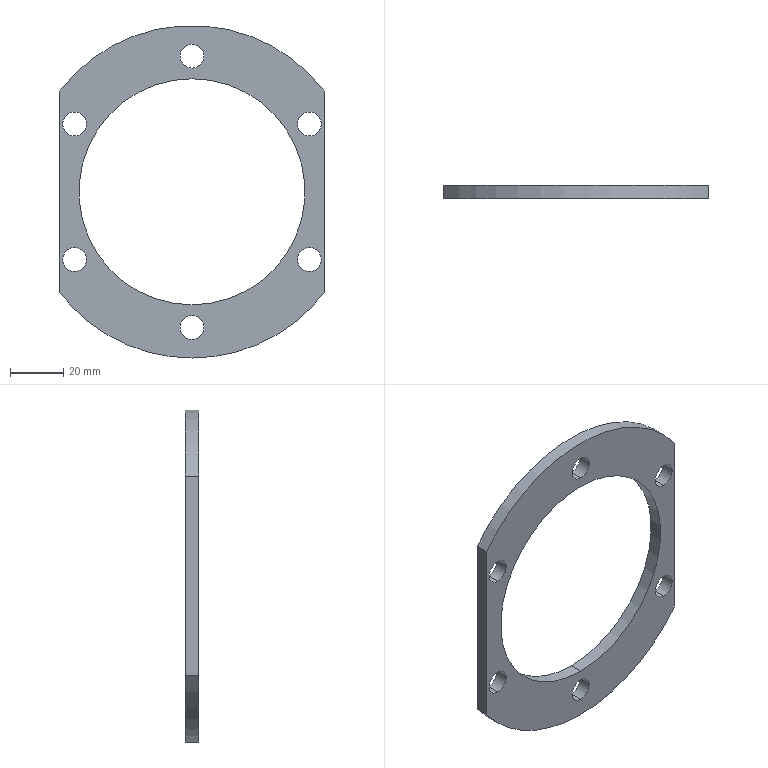Part | SolidWorks | features ICE 2, Extrusion 1 | 1 solid | 21 faces | box 100 x 5 x 125 mm | volume 24691 mm3 | cylinder 17 | plane 4 | commonest cylinder face diameters 9 x12 125 x3 85 x2
STEP:
#1=CARTESIAN_POINT('',(0.,0.,-55.5));
#2=VERTEX_POINT('',#1);
#3=CARTESIAN_POINT('',(0.,0.,-46.5));
#4=VERTEX_POINT('',#3);
#5=CARTESIAN_POINT('',(0.,0.,-51.));
#6=DIRECTION('',(0.,1.,0.));
#7=DIRECTION('',(0.,0.,1.));
#8=AXIS2_PLACEMENT_3D('',#5,#6,#7);
#9=CIRCLE('',#8,4.5);
#10=EDGE_CURVE('',#2,#4,#9,.T.);
#11=ORIENTED_EDGE('',*,*,#10,.F.);
#12=CARTESIAN_POINT('',(0.,5.,-55.5));
#13=VERTEX_POINT('',#12);
#14=CARTESIAN_POINT('',(0.,-5.,-55.5));
#15=DIRECTION('',(0.,1.,0.));
#16=VECTOR('',#15,1000.);
#17=LINE('',#14,#16);
#18=EDGE_CURVE('',#2,#13,#17,.T.);
#19=ORIENTED_EDGE('',*,*,#18,.T.);
#20=CARTESIAN_POINT('',(0.,5.,-46.5));
#21=VERTEX_POINT('',#20);
#22=CARTESIAN_POINT('',(0.,5.,-51.));
#23=DIRECTION('',(0.,1.,0.));
#24=DIRECTION('',(0.,0.,1.));
#25=AXIS2_PLACEMENT_3D('',#22,#23,#24);
#26=CIRCLE('',#25,4.5);
#27=EDGE_CURVE('',#13,#21,#26,.T.);
#28=ORIENTED_EDGE('',*,*,#27,.T.);
#29=CARTESIAN_POINT('',(0.,-5.,-46.5));
#30=DIRECTION('',(0.,1.,0.));
#31=VECTOR('',#30,1000.);
#32=LINE('',#29,#31);
#33=EDGE_CURVE('',#4,#21,#32,.T.);
#34=ORIENTED_EDGE('',*,*,#33,.F.);
#35=EDGE_LOOP('',(#11,#19,#28,#34));
#36=FACE_OUTER_BOUND('',#35,.T.);
#37=CARTESIAN_POINT('',(0.,-5.,-51.));
#38=DIRECTION('',(0.,1.,0.));
#39=DIRECTION('',(0.,0.,1.));
#40=AXIS2_PLACEMENT_3D('',#37,#38,#39);
#41=CYLINDRICAL_SURFACE('',#40,4.5);
#42=ADVANCED_FACE('',(#36),#41,.F.);
#43=CARTESIAN_POINT('',(-44.167,0.,-30.));
#44=VERTEX_POINT('',#43);
#45=CARTESIAN_POINT('',(-44.167,0.,-21.));
#46=VERTEX_POINT('',#45);
#47=CARTESIAN_POINT('',(-44.167,0.,-25.5));
#48=DIRECTION('',(0.,1.,0.));
#49=DIRECTION('',(0.,0.,1.));
#50=AXIS2_PLACEMENT_3D('',#47,#48,#49);
#51=CIRCLE('',#50,4.5);
#52=EDGE_CURVE('',#44,#46,#51,.T.);
#53=ORIENTED_EDGE('',*,*,#52,.F.);
#54=CARTESIAN_POINT('',(-44.167,5.,-30.));
#55=VERTEX_POINT('',#54);
#56=CARTESIAN_POINT('',(-44.167,-5.,-30.));
#57=DIRECTION('',(0.,1.,0.));
#58=VECTOR('',#57,1000.);
#59=LINE('',#56,#58);
#60=EDGE_CURVE('',#44,#55,#59,.T.);
#61=ORIENTED_EDGE('',*,*,#60,.T.);
#62=CARTESIAN_POINT('',(-44.167,5.,-21.));
#63=VERTEX_POINT('',#62);
#64=CARTESIAN_POINT('',(-44.167,5.,-25.5));
#65=DIRECTION('',(0.,1.,0.));
#66=DIRECTION('',(0.,0.,1.));
#67=AXIS2_PLACEMENT_3D('',#64,#65,#66);
#68=CIRCLE('',#67,4.5);
#69=EDGE_CURVE('',#55,#63,#68,.T.);
#70=ORIENTED_EDGE('',*,*,#69,.T.);
#71=CARTESIAN_POINT('',(-44.167,-5.,-21.));
#72=DIRECTION('',(0.,1.,0.));
#73=VECTOR('',#72,1000.);
#74=LINE('',#71,#73);
#75=EDGE_CURVE('',#46,#63,#74,.T.);
#76=ORIENTED_EDGE('',*,*,#75,.F.);
#77=EDGE_LOOP('',(#53,#61,#70,#76));
#78=FACE_OUTER_BOUND('',#77,.T.);
#79=CARTESIAN_POINT('',(-44.167,-5.,-25.5));
#80=DIRECTION('',(0.,1.,0.));
#81=DIRECTION('',(0.,0.,1.));
#82=AXIS2_PLACEMENT_3D('',#79,#80,#81);
#83=CYLINDRICAL_SURFACE('',#82,4.5);
#84=ADVANCED_FACE('',(#78),#83,.F.);
#85=CARTESIAN_POINT('',(-44.167,0.,21.));
#86=VERTEX_POINT('',#85);
#87=CARTESIAN_POINT('',(-44.167,0.,30.));
#88=VERTEX_POINT('',#87);
#89=CARTESIAN_POINT('',(-44.167,0.,25.5));
#90=DIRECTION('',(0.,1.,0.));
#91=DIRECTION('',(0.,0.,1.));
#92=AXIS2_PLACEMENT_3D('',#89,#90,#91);
#93=CIRCLE('',#92,4.5);
#94=EDGE_CURVE('',#86,#88,#93,.T.);
#95=ORIENTED_EDGE('',*,*,#94,.F.);
#96=CARTESIAN_POINT('',(-44.167,5.,21.));
#97=VERTEX_POINT('',#96);
#98=CARTESIAN_POINT('',(-44.167,-5.,21.));
#99=DIRECTION('',(0.,1.,0.));
#100=VECTOR('',#99,1000.);
#101=LINE('',#98,#100);
#102=EDGE_CURVE('',#86,#97,#101,.T.);
#103=ORIENTED_EDGE('',*,*,#102,.T.);
#104=CARTESIAN_POINT('',(-44.167,5.,30.));
#105=VERTEX_POINT('',#104);
#106=CARTESIAN_POINT('',(-44.167,5.,25.5));
#107=DIRECTION('',(0.,1.,0.));
#108=DIRECTION('',(0.,0.,1.));
#109=AXIS2_PLACEMENT_3D('',#106,#107,#108);
#110=CIRCLE('',#109,4.5);
#111=EDGE_CURVE('',#97,#105,#110,.T.);
#112=ORIENTED_EDGE('',*,*,#111,.T.);
#113=CARTESIAN_POINT('',(-44.167,-5.,30.));
#114=DIRECTION('',(0.,1.,0.));
#115=VECTOR('',#114,1000.);
#116=LINE('',#113,#115);
#117=EDGE_CURVE('',#88,#105,#116,.T.);
#118=ORIENTED_EDGE('',*,*,#117,.F.);
#119=EDGE_LOOP('',(#95,#103,#112,#118));
#120=FACE_OUTER_BOUND('',#119,.T.);
#121=CARTESIAN_POINT('',(-44.167,-5.,25.5));
#122=DIRECTION('',(0.,1.,0.));
#123=DIRECTION('',(0.,0.,1.));
#124=AXIS2_PLACEMENT_3D('',#121,#122,#123);
#125=CYLINDRICAL_SURFACE('',#124,4.5);
#126=ADVANCED_FACE('',(#120),#125,.F.);
#127=CARTESIAN_POINT('',(0.,0.,46.5));
#128=VERTEX_POINT('',#127);
#129=CARTESIAN_POINT('',(0.,0.,55.5));
#130=VERTEX_POINT('',#129);
#131=CARTESIAN_POINT('',(0.,0.,51.));
#132=DIRECTION('',(0.,1.,0.));
#133=DIRECTION('',(0.,0.,1.));
#134=AXIS2_PLACEMENT_3D('',#131,#132,#133);
#135=CIRCLE('',#134,4.5);
#136=EDGE_CURVE('',#128,#130,#135,.T.);
#137=ORIENTED_EDGE('',*,*,#136,.F.);
#138=CARTESIAN_POINT('',(0.,5.,46.5));
#139=VERTEX_POINT('',#138);
#140=CARTESIAN_POINT('',(0.,-5.,46.5));
#141=DIRECTION('',(0.,1.,0.));
#142=VECTOR('',#141,1000.);
#143=LINE('',#140,#142);
#144=EDGE_CURVE('',#128,#139,#143,.T.);
#145=ORIENTED_EDGE('',*,*,#144,.T.);
#146=CARTESIAN_POINT('',(0.,5.,55.5));
#147=VERTEX_POINT('',#146);
#148=CARTESIAN_POINT('',(0.,5.,51.));
#149=DIRECTION('',(0.,1.,0.));
#150=DIRECTION('',(0.,0.,1.));
#151=AXIS2_PLACEMENT_3D('',#148,#149,#150);
#152=CIRCLE('',#151,4.5);
#153=EDGE_CURVE('',#139,#147,#152,.T.);
#154=ORIENTED_EDGE('',*,*,#153,.T.);
#155=CARTESIAN_POINT('',(0.,-5.,55.5));
#156=DIRECTION('',(0.,1.,0.));
#157=VECTOR('',#156,1000.);
#158=LINE('',#155,#157);
#159=EDGE_CURVE('',#130,#147,#158,.T.);
#160=ORIENTED_EDGE('',*,*,#159,.F.);
#161=EDGE_LOOP('',(#137,#145,#154,#160));
#162=FACE_OUTER_BOUND('',#161,.T.);
#163=CARTESIAN_POINT('',(0.,-5.,51.));
#164=DIRECTION('',(0.,1.,0.));
#165=DIRECTION('',(0.,0.,1.));
#166=AXIS2_PLACEMENT_3D('',#163,#164,#165);
#167=CYLINDRICAL_SURFACE('',#166,4.5);
#168=ADVANCED_FACE('',(#162),#167,.F.);
#169=CARTESIAN_POINT('',(44.167,0.,21.));
#170=VERTEX_POINT('',#169);
#171=CARTESIAN_POINT('',(44.167,0.,30.));
#172=VERTEX_POINT('',#171);
#173=CARTESIAN_POINT('',(44.167,0.,25.5));
#174=DIRECTION('',(0.,1.,0.));
#175=DIRECTION('',(0.,0.,1.));
#176=AXIS2_PLACEMENT_3D('',#173,#174,#175);
#177=CIRCLE('',#176,4.5);
#178=EDGE_CURVE('',#170,#172,#177,.T.);
#179=ORIENTED_EDGE('',*,*,#178,.F.);
#180=CARTESIAN_POINT('',(44.167,5.,21.));
#181=VERTEX_POINT('',#180);
#182=CARTESIAN_POINT('',(44.167,-5.,21.));
#183=DIRECTION('',(0.,1.,0.));
#184=VECTOR('',#183,1000.);
#185=LINE('',#182,#184);
#186=EDGE_CURVE('',#170,#181,#185,.T.);
#187=ORIENTED_EDGE('',*,*,#186,.T.);
#188=CARTESIAN_POINT('',(44.167,5.,30.));
#189=VERTEX_POINT('',#188);
#190=CARTESIAN_POINT('',(44.167,5.,25.5));
#191=DIRECTION('',(0.,1.,0.));
#192=DIRECTION('',(0.,0.,1.));
#193=AXIS2_PLACEMENT_3D('',#190,#191,#192);
#194=CIRCLE('',#193,4.5);
#195=EDGE_CURVE('',#181,#189,#194,.T.);
#196=ORIENTED_EDGE('',*,*,#195,.T.);
#197=CARTESIAN_POINT('',(44.167,-5.,30.));
#198=DIRECTION('',(0.,1.,0.));
#199=VECTOR('',#198,1000.);
#200=LINE('',#197,#199);
#201=EDGE_CURVE('',#172,#189,#200,.T.);
#202=ORIENTED_EDGE('',*,*,#201,.F.);
#203=EDGE_LOOP('',(#179,#187,#196,#202));
#204=FACE_OUTER_BOUND('',#203,.T.);
#205=CARTESIAN_POINT('',(44.167,-5.,25.5));
#206=DIRECTION('',(0.,1.,0.));
#207=DIRECTION('',(0.,0.,1.));
#208=AXIS2_PLACEMENT_3D('',#205,#206,#207);
#209=CYLINDRICAL_SURFACE('',#208,4.5);
#210=ADVANCED_FACE('',(#204),#209,.F.);
#211=CARTESIAN_POINT('',(44.167,0.,-30.));
#212=VERTEX_POINT('',#211);
#213=CARTESIAN_POINT('',(44.167,0.,-21.));
#214=VERTEX_POINT('',#213);
#215=CARTESIAN_POINT('',(44.167,0.,-25.5));
#216=DIRECTION('',(0.,1.,0.));
#217=DIRECTION('',(0.,0.,1.));
#218=AXIS2_PLACEMENT_3D('',#215,#216,#217);
#219=CIRCLE('',#218,4.5);
#220=EDGE_CURVE('',#212,#214,#219,.T.);
#221=ORIENTED_EDGE('',*,*,#220,.F.);
#222=CARTESIAN_POINT('',(44.167,5.,-30.));
#223=VERTEX_POINT('',#222);
#224=CARTESIAN_POINT('',(44.167,-5.,-30.));
#225=DIRECTION('',(0.,1.,0.));
#226=VECTOR('',#225,1000.);
#227=LINE('',#224,#226);
#228=EDGE_CURVE('',#212,#223,#227,.T.);
#229=ORIENTED_EDGE('',*,*,#228,.T.);
#230=CARTESIAN_POINT('',(44.167,5.,-21.));
#231=VERTEX_POINT('',#230);
#232=CARTESIAN_POINT('',(44.167,5.,-25.5));
#233=DIRECTION('',(0.,1.,0.));
#234=DIRECTION('',(0.,0.,1.));
#235=AXIS2_PLACEMENT_3D('',#232,#233,#234);
#236=CIRCLE('',#235,4.5);
#237=EDGE_CURVE('',#223,#231,#236,.T.);
#238=ORIENTED_EDGE('',*,*,#237,.T.);
#239=CARTESIAN_POINT('',(44.167,-5.,-21.));
#240=DIRECTION('',(0.,1.,0.));
#241=VECTOR('',#240,1000.);
#242=LINE('',#239,#241);
#243=EDGE_CURVE('',#214,#231,#242,.T.);
#244=ORIENTED_EDGE('',*,*,#243,.F.);
#245=EDGE_LOOP('',(#221,#229,#238,#244));
#246=FACE_OUTER_BOUND('',#245,.T.);
#247=CARTESIAN_POINT('',(44.167,-5.,-25.5));
#248=DIRECTION('',(0.,1.,0.));
#249=DIRECTION('',(0.,0.,1.));
#250=AXIS2_PLACEMENT_3D('',#247,#248,#249);
#251=CYLINDRICAL_SURFACE('',#250,4.5);
#252=ADVANCED_FACE('',(#246),#251,.F.);
#253=CARTESIAN_POINT('',(0.,5.,-42.5));
#254=VERTEX_POINT('',#253);
#255=CARTESIAN_POINT('',(0.,5.,42.5));
#256=VERTEX_POINT('',#255);
#257=CARTESIAN_POINT('',(0.,5.,0.));
#258=DIRECTION('',(0.,1.,0.));
#259=DIRECTION('',(0.,0.,1.));
#260=AXIS2_PLACEMENT_3D('',#257,#258,#259);
#261=CIRCLE('',#260,42.5);
#262=EDGE_CURVE('',#254,#256,#261,.T.);
#263=ORIENTED_EDGE('',*,*,#262,.T.);
#264=CARTESIAN_POINT('',(0.,0.,42.5));
#265=VERTEX_POINT('',#264);
#266=CARTESIAN_POINT('',(0.,5.,42.5));
#267=DIRECTION('',(0.,-1.,0.));
#268=VECTOR('',#267,1000.);
#269=LINE('',#266,#268);
#270=EDGE_CURVE('',#256,#265,#269,.T.);
#271=ORIENTED_EDGE('',*,*,#270,.T.);
#272=CARTESIAN_POINT('',(0.,0.,-42.5));
#273=VERTEX_POINT('',#272);
#274=CARTESIAN_POINT('',(0.,0.,0.));
#275=DIRECTION('',(0.,1.,0.));
#276=DIRECTION('',(0.,0.,1.));
#277=AXIS2_PLACEMENT_3D('',#274,#275,#276);
#278=CIRCLE('',#277,42.5);
#279=EDGE_CURVE('',#273,#265,#278,.T.);
#280=ORIENTED_EDGE('',*,*,#279,.F.);
#281=CARTESIAN_POINT('',(0.,5.,-42.5));
#282=DIRECTION('',(0.,-1.,0.));
#283=VECTOR('',#282,1000.);
#284=LINE('',#281,#283);
#285=EDGE_CURVE('',#254,#273,#284,.T.);
#286=ORIENTED_EDGE('',*,*,#285,.F.);
#287=EDGE_LOOP('',(#263,#271,#280,#286));
#288=FACE_OUTER_BOUND('',#287,.T.);
#289=CARTESIAN_POINT('',(0.,5.,0.));
#290=DIRECTION('',(0.,-1.,0.));
#291=DIRECTION('',(0.,0.,-1.));
#292=AXIS2_PLACEMENT_3D('',#289,#290,#291);
#293=CYLINDRICAL_SURFACE('',#292,42.5);
#294=ADVANCED_FACE('',(#288),#293,.F.);
#295=CARTESIAN_POINT('',(0.,5.,-62.5));
#296=VERTEX_POINT('',#295);
#297=CARTESIAN_POINT('',(-50.,5.,-37.5));
#298=VERTEX_POINT('',#297);
#299=CARTESIAN_POINT('',(0.,5.,0.));
#300=DIRECTION('',(0.,1.,0.));
#301=DIRECTION('',(0.,0.,1.));
#302=AXIS2_PLACEMENT_3D('',#299,#300,#301);
#303=CIRCLE('',#302,62.5);
#304=EDGE_CURVE('',#296,#298,#303,.T.);
#305=ORIENTED_EDGE('',*,*,#304,.F.);
#306=CARTESIAN_POINT('',(0.,0.,-62.5));
#307=VERTEX_POINT('',#306);
#308=CARTESIAN_POINT('',(0.,5.,-62.5));
#309=DIRECTION('',(0.,-1.,0.));
#310=VECTOR('',#309,1000.);
#311=LINE('',#308,#310);
#312=EDGE_CURVE('',#296,#307,#311,.T.);
#313=ORIENTED_EDGE('',*,*,#312,.T.);
#314=CARTESIAN_POINT('',(-50.,0.,-37.5));
#315=VERTEX_POINT('',#314);
#316=CARTESIAN_POINT('',(0.,0.,0.));
#317=DIRECTION('',(0.,1.,0.));
#318=DIRECTION('',(0.,0.,1.));
#319=AXIS2_PLACEMENT_3D('',#316,#317,#318);
#320=CIRCLE('',#319,62.5);
#321=EDGE_CURVE('',#307,#315,#320,.T.);
#322=ORIENTED_EDGE('',*,*,#321,.T.);
#323=CARTESIAN_POINT('',(-50.,5.,-37.5));
#324=DIRECTION('',(0.,-1.,0.));
#325=VECTOR('',#324,1000.);
#326=LINE('',#323,#325);
#327=EDGE_CURVE('',#298,#315,#326,.T.);
#328=ORIENTED_EDGE('',*,*,#327,.F.);
#329=EDGE_LOOP('',(#305,#313,#322,#328));
#330=FACE_OUTER_BOUND('',#329,.T.);
#331=CARTESIAN_POINT('',(0.,5.,0.));
#332=DIRECTION('',(0.,-1.,0.));
#333=DIRECTION('',(0.,0.,-1.));
#334=AXIS2_PLACEMENT_3D('',#331,#332,#333);
#335=CYLINDRICAL_SURFACE('',#334,62.5);
#336=ADVANCED_FACE('',(#330),#335,.T.);
#337=CARTESIAN_POINT('',(0.,5.,-51.));
#338=DIRECTION('',(0.,1.,0.));
#339=DIRECTION('',(0.,0.,1.));
#340=AXIS2_PLACEMENT_3D('',#337,#338,#339);
#341=CIRCLE('',#340,4.5);
#342=EDGE_CURVE('',#21,#13,#341,.T.);
#343=ORIENTED_EDGE('',*,*,#342,.F.);
#344=ORIENTED_EDGE('',*,*,#27,.F.);
#345=EDGE_LOOP('',(#343,#344));
#346=FACE_BOUND('',#345,.T.);
#347=CARTESIAN_POINT('',(-44.167,5.,-25.5));
#348=DIRECTION('',(0.,1.,0.));
#349=DIRECTION('',(0.,0.,1.));
#350=AXIS2_PLACEMENT_3D('',#347,#348,#349);
#351=CIRCLE('',#350,4.5);
#352=EDGE_CURVE('',#63,#55,#351,.T.);
#353=ORIENTED_EDGE('',*,*,#352,.F.);
#354=ORIENTED_EDGE('',*,*,#69,.F.);
#355=EDGE_LOOP('',(#353,#354));
#356=FACE_BOUND('',#355,.T.);
#357=CARTESIAN_POINT('',(-44.167,5.,25.5));
#358=DIRECTION('',(0.,1.,0.));
#359=DIRECTION('',(0.,0.,1.));
#360=AXIS2_PLACEMENT_3D('',#357,#358,#359);
#361=CIRCLE('',#360,4.5);
#362=EDGE_CURVE('',#105,#97,#361,.T.);
#363=ORIENTED_EDGE('',*,*,#362,.F.);
#364=ORIENTED_EDGE('',*,*,#111,.F.);
#365=EDGE_LOOP('',(#363,#364));
#366=FACE_BOUND('',#365,.T.);
#367=CARTESIAN_POINT('',(0.,5.,51.));
#368=DIRECTION('',(0.,1.,0.));
#369=DIRECTION('',(0.,0.,1.));
#370=AXIS2_PLACEMENT_3D('',#367,#368,#369);
#371=CIRCLE('',#370,4.5);
#372=EDGE_CURVE('',#147,#139,#371,.T.);
#373=ORIENTED_EDGE('',*,*,#372,.F.);
#374=ORIENTED_EDGE('',*,*,#153,.F.);
#375=EDGE_LOOP('',(#373,#374));
#376=FACE_BOUND('',#375,.T.);
#377=CARTESIAN_POINT('',(44.167,5.,25.5));
#378=DIRECTION('',(0.,1.,0.));
#379=DIRECTION('',(0.,0.,1.));
#380=AXIS2_PLACEMENT_3D('',#377,#378,#379);
#381=CIRCLE('',#380,4.5);
#382=EDGE_CURVE('',#189,#181,#381,.T.);
#383=ORIENTED_EDGE('',*,*,#382,.F.);
#384=ORIENTED_EDGE('',*,*,#195,.F.);
#385=EDGE_LOOP('',(#383,#384));
#386=FACE_BOUND('',#385,.T.);
#387=CARTESIAN_POINT('',(44.167,5.,-25.5));
#388=DIRECTION('',(0.,1.,0.));
#389=DIRECTION('',(0.,0.,1.));
#390=AXIS2_PLACEMENT_3D('',#387,#388,#389);
#391=CIRCLE('',#390,4.5);
#392=EDGE_CURVE('',#231,#223,#391,.T.);
#393=ORIENTED_EDGE('',*,*,#392,.F.);
#394=ORIENTED_EDGE('',*,*,#237,.F.);
#395=EDGE_LOOP('',(#393,#394));
#396=FACE_BOUND('',#395,.T.);
#397=ORIENTED_EDGE('',*,*,#262,.F.);
#398=CARTESIAN_POINT('',(0.,5.,0.));
#399=DIRECTION('',(0.,1.,0.));
#400=DIRECTION('',(0.,0.,1.));
#401=AXIS2_PLACEMENT_3D('',#398,#399,#400);
#402=CIRCLE('',#401,42.5);
#403=EDGE_CURVE('',#256,#254,#402,.T.);
#404=ORIENTED_EDGE('',*,*,#403,.F.);
#405=EDGE_LOOP('',(#397,#404));
#406=FACE_BOUND('',#405,.T.);
#407=CARTESIAN_POINT('',(50.,5.,-37.5));
#408=VERTEX_POINT('',#407);
#409=CARTESIAN_POINT('',(0.,5.,0.));
#410=DIRECTION('',(0.,1.,0.));
#411=DIRECTION('',(0.,0.,1.));
#412=AXIS2_PLACEMENT_3D('',#409,#410,#411);
#413=CIRCLE('',#412,62.5);
#414=EDGE_CURVE('',#408,#296,#413,.T.);
#415=ORIENTED_EDGE('',*,*,#414,.T.);
#416=ORIENTED_EDGE('',*,*,#304,.T.);
#417=CARTESIAN_POINT('',(-50.,5.,37.5));
#418=VERTEX_POINT('',#417);
#419=CARTESIAN_POINT('',(-50.,5.,71.766));
#420=DIRECTION('',(0.,0.,1.));
#421=VECTOR('',#420,1000.);
#422=LINE('',#419,#421);
#423=EDGE_CURVE('',#298,#418,#422,.T.);
#424=ORIENTED_EDGE('',*,*,#423,.T.);
#425=CARTESIAN_POINT('',(50.,5.,37.5));
#426=VERTEX_POINT('',#425);
#427=CARTESIAN_POINT('',(0.,5.,0.));
#428=DIRECTION('',(0.,1.,0.));
#429=DIRECTION('',(0.,0.,1.));
#430=AXIS2_PLACEMENT_3D('',#427,#428,#429);
#431=CIRCLE('',#430,62.5);
#432=EDGE_CURVE('',#418,#426,#431,.T.);
#433=ORIENTED_EDGE('',*,*,#432,.T.);
#434=CARTESIAN_POINT('',(50.,5.,71.766));
#435=DIRECTION('',(0.,0.,-1.));
#436=VECTOR('',#435,1000.);
#437=LINE('',#434,#436);
#438=EDGE_CURVE('',#426,#408,#437,.T.);
#439=ORIENTED_EDGE('',*,*,#438,.T.);
#440=EDGE_LOOP('',(#415,#416,#424,#433,#439));
#441=FACE_OUTER_BOUND('',#440,.T.);
#442=CARTESIAN_POINT('',(0.,5.,0.));
#443=DIRECTION('',(0.,1.,0.));
#444=DIRECTION('',(0.,0.,1.));
#445=AXIS2_PLACEMENT_3D('',#442,#443,#444);
#446=PLANE('',#445);
#447=ADVANCED_FACE('',(#346,#356,#366,#376,#386,#396,#406,#441),#446,.T.);
#448=CARTESIAN_POINT('',(0.,0.,-51.));
#449=DIRECTION('',(0.,1.,0.));
#450=DIRECTION('',(0.,0.,1.));
#451=AXIS2_PLACEMENT_3D('',#448,#449,#450);
#452=CIRCLE('',#451,4.5);
#453=EDGE_CURVE('',#4,#2,#452,.T.);
#454=ORIENTED_EDGE('',*,*,#453,.T.);
#455=ORIENTED_EDGE('',*,*,#10,.T.);
#456=EDGE_LOOP('',(#454,#455));
#457=FACE_BOUND('',#456,.T.);
#458=CARTESIAN_POINT('',(-44.167,0.,-25.5));
#459=DIRECTION('',(0.,1.,0.));
#460=DIRECTION('',(0.,0.,1.));
#461=AXIS2_PLACEMENT_3D('',#458,#459,#460);
#462=CIRCLE('',#461,4.5);
#463=EDGE_CURVE('',#46,#44,#462,.T.);
#464=ORIENTED_EDGE('',*,*,#463,.T.);
#465=ORIENTED_EDGE('',*,*,#52,.T.);
#466=EDGE_LOOP('',(#464,#465));
#467=FACE_BOUND('',#466,.T.);
#468=CARTESIAN_POINT('',(-44.167,0.,25.5));
#469=DIRECTION('',(0.,1.,0.));
#470=DIRECTION('',(0.,0.,1.));
#471=AXIS2_PLACEMENT_3D('',#468,#469,#470);
#472=CIRCLE('',#471,4.5);
#473=EDGE_CURVE('',#88,#86,#472,.T.);
#474=ORIENTED_EDGE('',*,*,#473,.T.);
#475=ORIENTED_EDGE('',*,*,#94,.T.);
#476=EDGE_LOOP('',(#474,#475));
#477=FACE_BOUND('',#476,.T.);
#478=CARTESIAN_POINT('',(0.,0.,51.));
#479=DIRECTION('',(0.,1.,0.));
#480=DIRECTION('',(0.,0.,1.));
#481=AXIS2_PLACEMENT_3D('',#478,#479,#480);
#482=CIRCLE('',#481,4.5);
#483=EDGE_CURVE('',#130,#128,#482,.T.);
#484=ORIENTED_EDGE('',*,*,#483,.T.);
#485=ORIENTED_EDGE('',*,*,#136,.T.);
#486=EDGE_LOOP('',(#484,#485));
#487=FACE_BOUND('',#486,.T.);
#488=CARTESIAN_POINT('',(44.167,0.,25.5));
#489=DIRECTION('',(0.,1.,0.));
#490=DIRECTION('',(0.,0.,1.));
#491=AXIS2_PLACEMENT_3D('',#488,#489,#490);
#492=CIRCLE('',#491,4.5);
#493=EDGE_CURVE('',#172,#170,#492,.T.);
#494=ORIENTED_EDGE('',*,*,#493,.T.);
#495=ORIENTED_EDGE('',*,*,#178,.T.);
#496=EDGE_LOOP('',(#494,#495));
#497=FACE_BOUND('',#496,.T.);
#498=CARTESIAN_POINT('',(44.167,0.,-25.5));
#499=DIRECTION('',(0.,1.,0.));
#500=DIRECTION('',(0.,0.,1.));
#501=AXIS2_PLACEMENT_3D('',#498,#499,#500);
#502=CIRCLE('',#501,4.5);
#503=EDGE_CURVE('',#214,#212,#502,.T.);
#504=ORIENTED_EDGE('',*,*,#503,.T.);
#505=ORIENTED_EDGE('',*,*,#220,.T.);
#506=EDGE_LOOP('',(#504,#505));
#507=FACE_BOUND('',#506,.T.);
#508=ORIENTED_EDGE('',*,*,#279,.T.);
#509=CARTESIAN_POINT('',(0.,0.,0.));
#510=DIRECTION('',(0.,1.,0.));
#511=DIRECTION('',(0.,0.,1.));
#512=AXIS2_PLACEMENT_3D('',#509,#510,#511);
#513=CIRCLE('',#512,42.5);
#514=EDGE_CURVE('',#265,#273,#513,.T.);
#515=ORIENTED_EDGE('',*,*,#514,.T.);
#516=EDGE_LOOP('',(#508,#515));
#517=FACE_BOUND('',#516,.T.);
#518=CARTESIAN_POINT('',(-50.,0.,37.5));
#519=VERTEX_POINT('',#518);
#520=CARTESIAN_POINT('',(-50.,0.,0.));
#521=DIRECTION('',(0.,0.,1.));
#522=VECTOR('',#521,1000.);
#523=LINE('',#520,#522);
#524=EDGE_CURVE('',#315,#519,#523,.T.);
#525=ORIENTED_EDGE('',*,*,#524,.F.);
#526=ORIENTED_EDGE('',*,*,#321,.F.);
#527=CARTESIAN_POINT('',(50.,0.,-37.5));
#528=VERTEX_POINT('',#527);
#529=CARTESIAN_POINT('',(0.,0.,0.));
#530=DIRECTION('',(0.,1.,0.));
#531=DIRECTION('',(0.,0.,1.));
#532=AXIS2_PLACEMENT_3D('',#529,#530,#531);
#533=CIRCLE('',#532,62.5);
#534=EDGE_CURVE('',#528,#307,#533,.T.);
#535=ORIENTED_EDGE('',*,*,#534,.F.);
#536=CARTESIAN_POINT('',(50.,0.,37.5));
#537=VERTEX_POINT('',#536);
#538=CARTESIAN_POINT('',(50.,0.,0.));
#539=DIRECTION('',(0.,0.,-1.));
#540=VECTOR('',#539,1000.);
#541=LINE('',#538,#540);
#542=EDGE_CURVE('',#537,#528,#541,.T.);
#543=ORIENTED_EDGE('',*,*,#542,.F.);
#544=CARTESIAN_POINT('',(0.,0.,0.));
#545=DIRECTION('',(0.,1.,0.));
#546=DIRECTION('',(0.,0.,1.));
#547=AXIS2_PLACEMENT_3D('',#544,#545,#546);
#548=CIRCLE('',#547,62.5);
#549=EDGE_CURVE('',#519,#537,#548,.T.);
#550=ORIENTED_EDGE('',*,*,#549,.F.);
#551=EDGE_LOOP('',(#525,#526,#535,#543,#550));
#552=FACE_OUTER_BOUND('',#551,.T.);
#553=CARTESIAN_POINT('',(0.,0.,0.));
#554=DIRECTION('',(0.,1.,0.));
#555=DIRECTION('',(0.,0.,1.));
#556=AXIS2_PLACEMENT_3D('',#553,#554,#555);
#557=PLANE('',#556);
#558=ADVANCED_FACE('',(#457,#467,#477,#487,#497,#507,#517,#552),#557,.F.);
#559=ORIENTED_EDGE('',*,*,#312,.F.);
#560=ORIENTED_EDGE('',*,*,#414,.F.);
#561=CARTESIAN_POINT('',(50.,5.,-37.5));
#562=DIRECTION('',(0.,1.,0.));
#563=VECTOR('',#562,1000.);
#564=LINE('',#561,#563);
#565=EDGE_CURVE('',#528,#408,#564,.T.);
#566=ORIENTED_EDGE('',*,*,#565,.F.);
#567=ORIENTED_EDGE('',*,*,#534,.T.);
#568=EDGE_LOOP('',(#559,#560,#566,#567));
#569=FACE_OUTER_BOUND('',#568,.T.);
#570=CARTESIAN_POINT('',(0.,5.,0.));
#571=DIRECTION('',(0.,-1.,0.));
#572=DIRECTION('',(0.,0.,-1.));
#573=AXIS2_PLACEMENT_3D('',#570,#571,#572);
#574=CYLINDRICAL_SURFACE('',#573,62.5);
#575=ADVANCED_FACE('',(#569),#574,.T.);
#576=CARTESIAN_POINT('',(-50.,5.,37.5));
#577=DIRECTION('',(0.,1.,0.));
#578=VECTOR('',#577,1000.);
#579=LINE('',#576,#578);
#580=EDGE_CURVE('',#519,#418,#579,.T.);
#581=ORIENTED_EDGE('',*,*,#580,.F.);
#582=ORIENTED_EDGE('',*,*,#549,.T.);
#583=CARTESIAN_POINT('',(50.,5.,37.5));
#584=DIRECTION('',(0.,-1.,0.));
#585=VECTOR('',#584,1000.);
#586=LINE('',#583,#585);
#587=EDGE_CURVE('',#426,#537,#586,.T.);
#588=ORIENTED_EDGE('',*,*,#587,.F.);
#589=ORIENTED_EDGE('',*,*,#432,.F.);
#590=EDGE_LOOP('',(#581,#582,#588,#589));
#591=FACE_OUTER_BOUND('',#590,.T.);
#592=CARTESIAN_POINT('',(0.,5.,0.));
#593=DIRECTION('',(0.,-1.,0.));
#594=DIRECTION('',(0.,0.,-1.));
#595=AXIS2_PLACEMENT_3D('',#592,#593,#594);
#596=CYLINDRICAL_SURFACE('',#595,62.5);
#597=ADVANCED_FACE('',(#591),#596,.T.);
#598=ORIENTED_EDGE('',*,*,#270,.F.);
#599=ORIENTED_EDGE('',*,*,#403,.T.);
#600=ORIENTED_EDGE('',*,*,#285,.T.);
#601=ORIENTED_EDGE('',*,*,#514,.F.);
#602=EDGE_LOOP('',(#598,#599,#600,#601));
#603=FACE_OUTER_BOUND('',#602,.T.);
#604=CARTESIAN_POINT('',(0.,5.,0.));
#605=DIRECTION('',(0.,-1.,0.));
#606=DIRECTION('',(0.,0.,-1.));
#607=AXIS2_PLACEMENT_3D('',#604,#605,#606);
#608=CYLINDRICAL_SURFACE('',#607,42.5);
#609=ADVANCED_FACE('',(#603),#608,.F.);
#610=ORIENTED_EDGE('',*,*,#228,.F.);
#611=ORIENTED_EDGE('',*,*,#503,.F.);
#612=ORIENTED_EDGE('',*,*,#243,.T.);
#613=ORIENTED_EDGE('',*,*,#392,.T.);
#614=EDGE_LOOP('',(#610,#611,#612,#613));
#615=FACE_OUTER_BOUND('',#614,.T.);
#616=CARTESIAN_POINT('',(44.167,-5.,-25.5));
#617=DIRECTION('',(0.,1.,0.));
#618=DIRECTION('',(0.,0.,1.));
#619=AXIS2_PLACEMENT_3D('',#616,#617,#618);
#620=CYLINDRICAL_SURFACE('',#619,4.5);
#621=ADVANCED_FACE('',(#615),#620,.F.);
#622=ORIENTED_EDGE('',*,*,#186,.F.);
#623=ORIENTED_EDGE('',*,*,#493,.F.);
#624=ORIENTED_EDGE('',*,*,#201,.T.);
#625=ORIENTED_EDGE('',*,*,#382,.T.);
#626=EDGE_LOOP('',(#622,#623,#624,#625));
#627=FACE_OUTER_BOUND('',#626,.T.);
#628=CARTESIAN_POINT('',(44.167,-5.,25.5));
#629=DIRECTION('',(0.,1.,0.));
#630=DIRECTION('',(0.,0.,1.));
#631=AXIS2_PLACEMENT_3D('',#628,#629,#630);
#632=CYLINDRICAL_SURFACE('',#631,4.5);
#633=ADVANCED_FACE('',(#627),#632,.F.);
#634=ORIENTED_EDGE('',*,*,#144,.F.);
#635=ORIENTED_EDGE('',*,*,#483,.F.);
#636=ORIENTED_EDGE('',*,*,#159,.T.);
#637=ORIENTED_EDGE('',*,*,#372,.T.);
#638=EDGE_LOOP('',(#634,#635,#636,#637));
#639=FACE_OUTER_BOUND('',#638,.T.);
#640=CARTESIAN_POINT('',(0.,-5.,51.));
#641=DIRECTION('',(0.,1.,0.));
#642=DIRECTION('',(0.,0.,1.));
#643=AXIS2_PLACEMENT_3D('',#640,#641,#642);
#644=CYLINDRICAL_SURFACE('',#643,4.5);
#645=ADVANCED_FACE('',(#639),#644,.F.);
#646=ORIENTED_EDGE('',*,*,#102,.F.);
#647=ORIENTED_EDGE('',*,*,#473,.F.);
#648=ORIENTED_EDGE('',*,*,#117,.T.);
#649=ORIENTED_EDGE('',*,*,#362,.T.);
#650=EDGE_LOOP('',(#646,#647,#648,#649));
#651=FACE_OUTER_BOUND('',#650,.T.);
#652=CARTESIAN_POINT('',(-44.167,-5.,25.5));
#653=DIRECTION('',(0.,1.,0.));
#654=DIRECTION('',(0.,0.,1.));
#655=AXIS2_PLACEMENT_3D('',#652,#653,#654);
#656=CYLINDRICAL_SURFACE('',#655,4.5);
#657=ADVANCED_FACE('',(#651),#656,.F.);
#658=ORIENTED_EDGE('',*,*,#60,.F.);
#659=ORIENTED_EDGE('',*,*,#463,.F.);
#660=ORIENTED_EDGE('',*,*,#75,.T.);
#661=ORIENTED_EDGE('',*,*,#352,.T.);
#662=EDGE_LOOP('',(#658,#659,#660,#661));
#663=FACE_OUTER_BOUND('',#662,.T.);
#664=CARTESIAN_POINT('',(-44.167,-5.,-25.5));
#665=DIRECTION('',(0.,1.,0.));
#666=DIRECTION('',(0.,0.,1.));
#667=AXIS2_PLACEMENT_3D('',#664,#665,#666);
#668=CYLINDRICAL_SURFACE('',#667,4.5);
#669=ADVANCED_FACE('',(#663),#668,.F.);
#670=ORIENTED_EDGE('',*,*,#18,.F.);
#671=ORIENTED_EDGE('',*,*,#453,.F.);
#672=ORIENTED_EDGE('',*,*,#33,.T.);
#673=ORIENTED_EDGE('',*,*,#342,.T.);
#674=EDGE_LOOP('',(#670,#671,#672,#673));
#675=FACE_OUTER_BOUND('',#674,.T.);
#676=CARTESIAN_POINT('',(0.,-5.,-51.));
#677=DIRECTION('',(0.,1.,0.));
#678=DIRECTION('',(0.,0.,1.));
#679=AXIS2_PLACEMENT_3D('',#676,#677,#678);
#680=CYLINDRICAL_SURFACE('',#679,4.5);
#681=ADVANCED_FACE('',(#675),#680,.F.);
#682=ORIENTED_EDGE('',*,*,#587,.T.);
#683=ORIENTED_EDGE('',*,*,#542,.T.);
#684=ORIENTED_EDGE('',*,*,#565,.T.);
#685=ORIENTED_EDGE('',*,*,#438,.F.);
#686=EDGE_LOOP('',(#682,#683,#684,#685));
#687=FACE_OUTER_BOUND('',#686,.T.);
#688=CARTESIAN_POINT('',(50.,-5.,71.766));
#689=DIRECTION('',(1.,0.,0.));
#690=DIRECTION('',(0.,0.,-1.));
#691=AXIS2_PLACEMENT_3D('',#688,#689,#690);
#692=PLANE('',#691);
#693=ADVANCED_FACE('',(#687),#692,.T.);
#694=ORIENTED_EDGE('',*,*,#327,.T.);
#695=ORIENTED_EDGE('',*,*,#524,.T.);
#696=ORIENTED_EDGE('',*,*,#580,.T.);
#697=ORIENTED_EDGE('',*,*,#423,.F.);
#698=EDGE_LOOP('',(#694,#695,#696,#697));
#699=FACE_OUTER_BOUND('',#698,.T.);
#700=CARTESIAN_POINT('',(-50.,-5.,71.766));
#701=DIRECTION('',(-1.,0.,0.));
#702=DIRECTION('',(0.,0.,1.));
#703=AXIS2_PLACEMENT_3D('',#700,#701,#702);
#704=PLANE('',#703);
#705=ADVANCED_FACE('',(#699),#704,.T.);
#706=CLOSED_SHELL('',(#42,#84,#126,#168,#210,#252,#294,#336,#447,#558,#575,#597,#609,#621,#633,#645,#657,#669,#681,#693,#705));
#707=MANIFOLD_SOLID_BREP('',#706);
#708=CARTESIAN_POINT('',(0.,0.,0.));
#709=DIRECTION('',(0.,0.,1.));
#710=DIRECTION('',(1.,0.,0.));
#711=AXIS2_PLACEMENT_3D('',#708,#709,#710);
#712=(LENGTH_UNIT()NAMED_UNIT(*)SI_UNIT(.MILLI.,.METRE.));
#713=UNCERTAINTY_MEASURE_WITH_UNIT(LENGTH_MEASURE(0.00001),#712,'','');
#714=(NAMED_UNIT(*)PLANE_ANGLE_UNIT()SI_UNIT($,.RADIAN.));
#715=(NAMED_UNIT(*)SI_UNIT($,.STERADIAN.)SOLID_ANGLE_UNIT());
#716=(GEOMETRIC_REPRESENTATION_CONTEXT(3)GLOBAL_UNCERTAINTY_ASSIGNED_CONTEXT((#713))GLOBAL_UNIT_ASSIGNED_CONTEXT((#712,#714,#715))REPRESENTATION_CONTEXT('',''));
#717=ADVANCED_BREP_SHAPE_REPRESENTATION('',(#707,#711),#716);